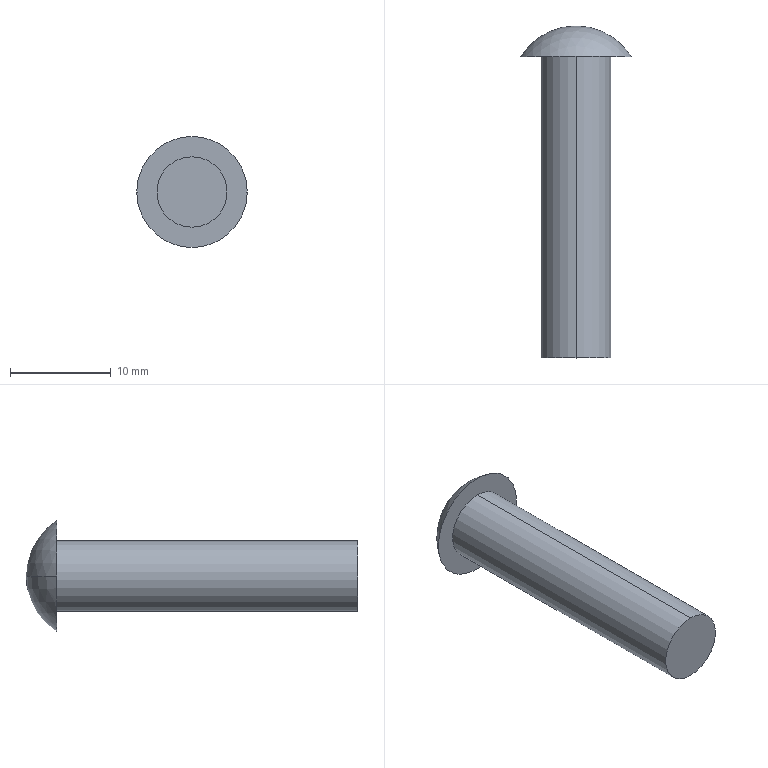Part | SolidWorks | features Revolution 1 | 1 solid | 6 faces | box 11 x 33 x 11 mm | volume 1312 mm3 | sphere 2 | cylinder 2 | plane 2 | commonest cylinder face diameters 7 x2
STEP:
#1=CARTESIAN_POINT('',(0.,18.,0.));
#2=VERTEX_POINT('',#1);
#3=CARTESIAN_POINT('',(5.5,14.961,0.));
#4=VERTEX_POINT('',#3);
#5=CARTESIAN_POINT('',(0.,11.503,0.));
#6=DIRECTION('',(0.,0.,-1.));
#7=DIRECTION('',(-1.,0.,0.));
#8=AXIS2_PLACEMENT_3D('',#5,#6,#7);
#9=CIRCLE('',#8,6.497);
#10=EDGE_CURVE('',#2,#4,#9,.T.);
#11=ORIENTED_EDGE('',*,*,#10,.F.);
#12=CARTESIAN_POINT('',(-5.5,14.961,0.));
#13=VERTEX_POINT('',#12);
#14=CARTESIAN_POINT('',(0.,11.503,0.));
#15=DIRECTION('',(0.,0.,1.));
#16=DIRECTION('',(1.,0.,0.));
#17=AXIS2_PLACEMENT_3D('',#14,#15,#16);
#18=CIRCLE('',#17,6.497);
#19=EDGE_CURVE('',#2,#13,#18,.T.);
#20=ORIENTED_EDGE('',*,*,#19,.T.);
#21=CARTESIAN_POINT('',(0.,14.961,0.));
#22=DIRECTION('',(0.,-1.,0.));
#23=DIRECTION('',(0.,0.,-1.));
#24=AXIS2_PLACEMENT_3D('',#21,#22,#23);
#25=CIRCLE('',#24,5.5);
#26=EDGE_CURVE('',#4,#13,#25,.T.);
#27=ORIENTED_EDGE('',*,*,#26,.F.);
#28=EDGE_LOOP('',(#11,#20,#27));
#29=FACE_OUTER_BOUND('',#28,.T.);
#30=CARTESIAN_POINT('',(0.,11.503,0.));
#31=DIRECTION('',(0.,0.,1.));
#32=DIRECTION('',(1.,0.,0.));
#33=AXIS2_PLACEMENT_3D('',#30,#31,#32);
#34=SPHERICAL_SURFACE('',#33,6.497);
#35=ADVANCED_FACE('',(#29),#34,.T.);
#36=CARTESIAN_POINT('',(0.,14.961,-3.5));
#37=VERTEX_POINT('',#36);
#38=CARTESIAN_POINT('',(0.,14.961,3.5));
#39=VERTEX_POINT('',#38);
#40=CARTESIAN_POINT('',(0.,14.961,0.));
#41=DIRECTION('',(0.,-1.,0.));
#42=DIRECTION('',(0.,0.,-1.));
#43=AXIS2_PLACEMENT_3D('',#40,#41,#42);
#44=CIRCLE('',#43,3.5);
#45=EDGE_CURVE('',#37,#39,#44,.T.);
#46=ORIENTED_EDGE('',*,*,#45,.T.);
#47=CARTESIAN_POINT('',(0.,-15.,3.5));
#48=VERTEX_POINT('',#47);
#49=CARTESIAN_POINT('',(0.,-15.,3.5));
#50=DIRECTION('',(0.,-1.,0.));
#51=VECTOR('',#50,1000.);
#52=LINE('',#49,#51);
#53=EDGE_CURVE('',#39,#48,#52,.T.);
#54=ORIENTED_EDGE('',*,*,#53,.T.);
#55=CARTESIAN_POINT('',(0.,-15.,-3.5));
#56=VERTEX_POINT('',#55);
#57=CARTESIAN_POINT('',(0.,-15.,0.));
#58=DIRECTION('',(0.,-1.,0.));
#59=DIRECTION('',(0.,0.,-1.));
#60=AXIS2_PLACEMENT_3D('',#57,#58,#59);
#61=CIRCLE('',#60,3.5);
#62=EDGE_CURVE('',#56,#48,#61,.T.);
#63=ORIENTED_EDGE('',*,*,#62,.F.);
#64=CARTESIAN_POINT('',(0.,-15.,-3.5));
#65=DIRECTION('',(0.,-1.,0.));
#66=VECTOR('',#65,1000.);
#67=LINE('',#64,#66);
#68=EDGE_CURVE('',#37,#56,#67,.T.);
#69=ORIENTED_EDGE('',*,*,#68,.F.);
#70=EDGE_LOOP('',(#46,#54,#63,#69));
#71=FACE_OUTER_BOUND('',#70,.T.);
#72=CARTESIAN_POINT('',(0.,-15.,0.));
#73=DIRECTION('',(0.,-1.,0.));
#74=DIRECTION('',(0.,0.,-1.));
#75=AXIS2_PLACEMENT_3D('',#72,#73,#74);
#76=CYLINDRICAL_SURFACE('',#75,3.5);
#77=ADVANCED_FACE('',(#71),#76,.T.);
#78=ORIENTED_EDGE('',*,*,#26,.T.);
#79=CARTESIAN_POINT('',(0.,14.961,0.));
#80=DIRECTION('',(0.,-1.,0.));
#81=DIRECTION('',(0.,0.,-1.));
#82=AXIS2_PLACEMENT_3D('',#79,#80,#81);
#83=CIRCLE('',#82,5.5);
#84=EDGE_CURVE('',#13,#4,#83,.T.);
#85=ORIENTED_EDGE('',*,*,#84,.T.);
#86=EDGE_LOOP('',(#78,#85));
#87=FACE_OUTER_BOUND('',#86,.T.);
#88=ORIENTED_EDGE('',*,*,#45,.F.);
#89=CARTESIAN_POINT('',(0.,14.961,0.));
#90=DIRECTION('',(0.,-1.,0.));
#91=DIRECTION('',(0.,0.,-1.));
#92=AXIS2_PLACEMENT_3D('',#89,#90,#91);
#93=CIRCLE('',#92,3.5);
#94=EDGE_CURVE('',#39,#37,#93,.T.);
#95=ORIENTED_EDGE('',*,*,#94,.F.);
#96=EDGE_LOOP('',(#88,#95));
#97=FACE_BOUND('',#96,.T.);
#98=CARTESIAN_POINT('',(3.5,14.961,0.));
#99=DIRECTION('',(0.,-1.,0.));
#100=DIRECTION('',(0.,0.,-1.));
#101=AXIS2_PLACEMENT_3D('',#98,#99,#100);
#102=PLANE('',#101);
#103=ADVANCED_FACE('',(#87,#97),#102,.T.);
#104=ORIENTED_EDGE('',*,*,#53,.F.);
#105=ORIENTED_EDGE('',*,*,#94,.T.);
#106=ORIENTED_EDGE('',*,*,#68,.T.);
#107=CARTESIAN_POINT('',(0.,-15.,0.));
#108=DIRECTION('',(0.,-1.,0.));
#109=DIRECTION('',(0.,0.,-1.));
#110=AXIS2_PLACEMENT_3D('',#107,#108,#109);
#111=CIRCLE('',#110,3.5);
#112=EDGE_CURVE('',#48,#56,#111,.T.);
#113=ORIENTED_EDGE('',*,*,#112,.F.);
#114=EDGE_LOOP('',(#104,#105,#106,#113));
#115=FACE_OUTER_BOUND('',#114,.T.);
#116=CARTESIAN_POINT('',(0.,-15.,0.));
#117=DIRECTION('',(0.,-1.,0.));
#118=DIRECTION('',(0.,0.,-1.));
#119=AXIS2_PLACEMENT_3D('',#116,#117,#118);
#120=CYLINDRICAL_SURFACE('',#119,3.5);
#121=ADVANCED_FACE('',(#115),#120,.T.);
#122=ORIENTED_EDGE('',*,*,#62,.T.);
#123=ORIENTED_EDGE('',*,*,#112,.T.);
#124=EDGE_LOOP('',(#122,#123));
#125=FACE_OUTER_BOUND('',#124,.T.);
#126=CARTESIAN_POINT('',(3.5,-15.,0.));
#127=DIRECTION('',(0.,-1.,0.));
#128=DIRECTION('',(0.,0.,-1.));
#129=AXIS2_PLACEMENT_3D('',#126,#127,#128);
#130=PLANE('',#129);
#131=ADVANCED_FACE('',(#125),#130,.T.);
#132=ORIENTED_EDGE('',*,*,#19,.F.);
#133=ORIENTED_EDGE('',*,*,#10,.T.);
#134=ORIENTED_EDGE('',*,*,#84,.F.);
#135=EDGE_LOOP('',(#132,#133,#134));
#136=FACE_OUTER_BOUND('',#135,.T.);
#137=CARTESIAN_POINT('',(0.,11.503,0.));
#138=DIRECTION('',(0.,0.,1.));
#139=DIRECTION('',(1.,0.,0.));
#140=AXIS2_PLACEMENT_3D('',#137,#138,#139);
#141=SPHERICAL_SURFACE('',#140,6.497);
#142=ADVANCED_FACE('',(#136),#141,.T.);
#143=CLOSED_SHELL('',(#35,#77,#103,#121,#131,#142));
#144=MANIFOLD_SOLID_BREP('',#143);
#145=CARTESIAN_POINT('',(0.,0.,0.));
#146=DIRECTION('',(0.,0.,1.));
#147=DIRECTION('',(1.,0.,0.));
#148=AXIS2_PLACEMENT_3D('',#145,#146,#147);
#149=(LENGTH_UNIT()NAMED_UNIT(*)SI_UNIT(.MILLI.,.METRE.));
#150=UNCERTAINTY_MEASURE_WITH_UNIT(LENGTH_MEASURE(0.00001),#149,'','');
#151=(NAMED_UNIT(*)PLANE_ANGLE_UNIT()SI_UNIT($,.RADIAN.));
#152=(NAMED_UNIT(*)SI_UNIT($,.STERADIAN.)SOLID_ANGLE_UNIT());
#153=(GEOMETRIC_REPRESENTATION_CONTEXT(3)GLOBAL_UNCERTAINTY_ASSIGNED_CONTEXT((#150))GLOBAL_UNIT_ASSIGNED_CONTEXT((#149,#151,#152))REPRESENTATION_CONTEXT('',''));
#154=ADVANCED_BREP_SHAPE_REPRESENTATION('',(#144,#148),#153);